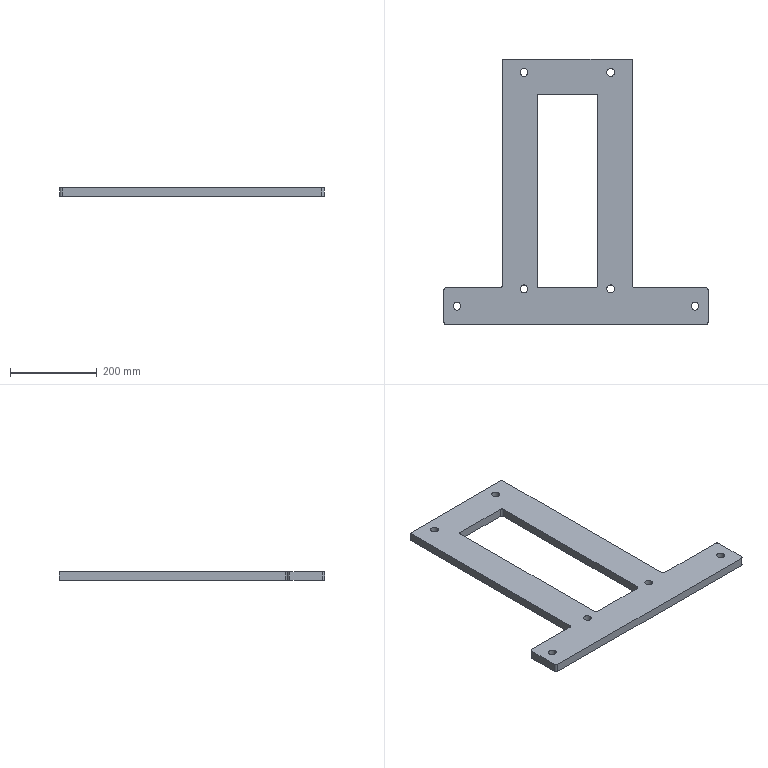Part | SolidWorks | features Extrusion 1 | 1 solid | 36 faces | box 610 x 612.5 x 20 mm | volume 2918678 mm3 | cylinder 22 | plane 14 | commonest cylinder face diameters 18 x12 10 x10
STEP:
#1=CARTESIAN_POINT('',(376.,82.5,20.));
#2=VERTEX_POINT('',#1);
#3=CARTESIAN_POINT('',(394.,82.5,20.));
#4=VERTEX_POINT('',#3);
#5=CARTESIAN_POINT('',(385.,82.5,20.));
#6=DIRECTION('',(0.,0.,1.));
#7=DIRECTION('',(1.,0.,0.));
#8=AXIS2_PLACEMENT_3D('',#5,#6,#7);
#9=CIRCLE('',#8,9.);
#10=EDGE_CURVE('',#2,#4,#9,.T.);
#11=ORIENTED_EDGE('',*,*,#10,.T.);
#12=CARTESIAN_POINT('',(394.,82.5,0.));
#13=VERTEX_POINT('',#12);
#14=CARTESIAN_POINT('',(394.,82.5,20.));
#15=DIRECTION('',(0.,0.,-1.));
#16=VECTOR('',#15,1000.);
#17=LINE('',#14,#16);
#18=EDGE_CURVE('',#4,#13,#17,.T.);
#19=ORIENTED_EDGE('',*,*,#18,.T.);
#20=CARTESIAN_POINT('',(376.,82.5,0.));
#21=VERTEX_POINT('',#20);
#22=CARTESIAN_POINT('',(385.,82.5,0.));
#23=DIRECTION('',(0.,0.,1.));
#24=DIRECTION('',(1.,0.,0.));
#25=AXIS2_PLACEMENT_3D('',#22,#23,#24);
#26=CIRCLE('',#25,9.);
#27=EDGE_CURVE('',#21,#13,#26,.T.);
#28=ORIENTED_EDGE('',*,*,#27,.F.);
#29=CARTESIAN_POINT('',(376.,82.5,20.));
#30=DIRECTION('',(0.,0.,-1.));
#31=VECTOR('',#30,1000.);
#32=LINE('',#29,#31);
#33=EDGE_CURVE('',#2,#21,#32,.T.);
#34=ORIENTED_EDGE('',*,*,#33,.F.);
#35=EDGE_LOOP('',(#11,#19,#28,#34));
#36=FACE_OUTER_BOUND('',#35,.T.);
#37=CARTESIAN_POINT('',(385.,82.5,20.));
#38=DIRECTION('',(0.,0.,-1.));
#39=DIRECTION('',(-1.,0.,0.));
#40=AXIS2_PLACEMENT_3D('',#37,#38,#39);
#41=CYLINDRICAL_SURFACE('',#40,9.);
#42=ADVANCED_FACE('',(#36),#41,.F.);
#43=CARTESIAN_POINT('',(176.,82.5,20.));
#44=VERTEX_POINT('',#43);
#45=CARTESIAN_POINT('',(194.,82.5,20.));
#46=VERTEX_POINT('',#45);
#47=CARTESIAN_POINT('',(185.,82.5,20.));
#48=DIRECTION('',(0.,0.,1.));
#49=DIRECTION('',(1.,0.,0.));
#50=AXIS2_PLACEMENT_3D('',#47,#48,#49);
#51=CIRCLE('',#50,9.);
#52=EDGE_CURVE('',#44,#46,#51,.T.);
#53=ORIENTED_EDGE('',*,*,#52,.T.);
#54=CARTESIAN_POINT('',(194.,82.5,0.));
#55=VERTEX_POINT('',#54);
#56=CARTESIAN_POINT('',(194.,82.5,20.));
#57=DIRECTION('',(0.,0.,-1.));
#58=VECTOR('',#57,1000.);
#59=LINE('',#56,#58);
#60=EDGE_CURVE('',#46,#55,#59,.T.);
#61=ORIENTED_EDGE('',*,*,#60,.T.);
#62=CARTESIAN_POINT('',(176.,82.5,0.));
#63=VERTEX_POINT('',#62);
#64=CARTESIAN_POINT('',(185.,82.5,0.));
#65=DIRECTION('',(0.,0.,1.));
#66=DIRECTION('',(1.,0.,0.));
#67=AXIS2_PLACEMENT_3D('',#64,#65,#66);
#68=CIRCLE('',#67,9.);
#69=EDGE_CURVE('',#63,#55,#68,.T.);
#70=ORIENTED_EDGE('',*,*,#69,.F.);
#71=CARTESIAN_POINT('',(176.,82.5,20.));
#72=DIRECTION('',(0.,0.,-1.));
#73=VECTOR('',#72,1000.);
#74=LINE('',#71,#73);
#75=EDGE_CURVE('',#44,#63,#74,.T.);
#76=ORIENTED_EDGE('',*,*,#75,.F.);
#77=EDGE_LOOP('',(#53,#61,#70,#76));
#78=FACE_OUTER_BOUND('',#77,.T.);
#79=CARTESIAN_POINT('',(185.,82.5,20.));
#80=DIRECTION('',(0.,0.,-1.));
#81=DIRECTION('',(-1.,0.,0.));
#82=AXIS2_PLACEMENT_3D('',#79,#80,#81);
#83=CYLINDRICAL_SURFACE('',#82,9.);
#84=ADVANCED_FACE('',(#78),#83,.F.);
#85=CARTESIAN_POINT('',(376.,582.5,20.));
#86=VERTEX_POINT('',#85);
#87=CARTESIAN_POINT('',(394.,582.5,20.));
#88=VERTEX_POINT('',#87);
#89=CARTESIAN_POINT('',(385.,582.5,20.));
#90=DIRECTION('',(0.,0.,1.));
#91=DIRECTION('',(1.,0.,0.));
#92=AXIS2_PLACEMENT_3D('',#89,#90,#91);
#93=CIRCLE('',#92,9.);
#94=EDGE_CURVE('',#86,#88,#93,.T.);
#95=ORIENTED_EDGE('',*,*,#94,.T.);
#96=CARTESIAN_POINT('',(394.,582.5,0.));
#97=VERTEX_POINT('',#96);
#98=CARTESIAN_POINT('',(394.,582.5,20.));
#99=DIRECTION('',(0.,0.,-1.));
#100=VECTOR('',#99,1000.);
#101=LINE('',#98,#100);
#102=EDGE_CURVE('',#88,#97,#101,.T.);
#103=ORIENTED_EDGE('',*,*,#102,.T.);
#104=CARTESIAN_POINT('',(376.,582.5,0.));
#105=VERTEX_POINT('',#104);
#106=CARTESIAN_POINT('',(385.,582.5,0.));
#107=DIRECTION('',(0.,0.,1.));
#108=DIRECTION('',(1.,0.,0.));
#109=AXIS2_PLACEMENT_3D('',#106,#107,#108);
#110=CIRCLE('',#109,9.);
#111=EDGE_CURVE('',#105,#97,#110,.T.);
#112=ORIENTED_EDGE('',*,*,#111,.F.);
#113=CARTESIAN_POINT('',(376.,582.5,20.));
#114=DIRECTION('',(0.,0.,-1.));
#115=VECTOR('',#114,1000.);
#116=LINE('',#113,#115);
#117=EDGE_CURVE('',#86,#105,#116,.T.);
#118=ORIENTED_EDGE('',*,*,#117,.F.);
#119=EDGE_LOOP('',(#95,#103,#112,#118));
#120=FACE_OUTER_BOUND('',#119,.T.);
#121=CARTESIAN_POINT('',(385.,582.5,20.));
#122=DIRECTION('',(0.,0.,-1.));
#123=DIRECTION('',(-1.,0.,0.));
#124=AXIS2_PLACEMENT_3D('',#121,#122,#123);
#125=CYLINDRICAL_SURFACE('',#124,9.);
#126=ADVANCED_FACE('',(#120),#125,.F.);
#127=CARTESIAN_POINT('',(176.,582.5,20.));
#128=VERTEX_POINT('',#127);
#129=CARTESIAN_POINT('',(194.,582.5,20.));
#130=VERTEX_POINT('',#129);
#131=CARTESIAN_POINT('',(185.,582.5,20.));
#132=DIRECTION('',(0.,0.,1.));
#133=DIRECTION('',(1.,0.,0.));
#134=AXIS2_PLACEMENT_3D('',#131,#132,#133);
#135=CIRCLE('',#134,9.);
#136=EDGE_CURVE('',#128,#130,#135,.T.);
#137=ORIENTED_EDGE('',*,*,#136,.T.);
#138=CARTESIAN_POINT('',(194.,582.5,0.));
#139=VERTEX_POINT('',#138);
#140=CARTESIAN_POINT('',(194.,582.5,20.));
#141=DIRECTION('',(0.,0.,-1.));
#142=VECTOR('',#141,1000.);
#143=LINE('',#140,#142);
#144=EDGE_CURVE('',#130,#139,#143,.T.);
#145=ORIENTED_EDGE('',*,*,#144,.T.);
#146=CARTESIAN_POINT('',(176.,582.5,0.));
#147=VERTEX_POINT('',#146);
#148=CARTESIAN_POINT('',(185.,582.5,0.));
#149=DIRECTION('',(0.,0.,1.));
#150=DIRECTION('',(1.,0.,0.));
#151=AXIS2_PLACEMENT_3D('',#148,#149,#150);
#152=CIRCLE('',#151,9.);
#153=EDGE_CURVE('',#147,#139,#152,.T.);
#154=ORIENTED_EDGE('',*,*,#153,.F.);
#155=CARTESIAN_POINT('',(176.,582.5,20.));
#156=DIRECTION('',(0.,0.,-1.));
#157=VECTOR('',#156,1000.);
#158=LINE('',#155,#157);
#159=EDGE_CURVE('',#128,#147,#158,.T.);
#160=ORIENTED_EDGE('',*,*,#159,.F.);
#161=EDGE_LOOP('',(#137,#145,#154,#160));
#162=FACE_OUTER_BOUND('',#161,.T.);
#163=CARTESIAN_POINT('',(185.,582.5,20.));
#164=DIRECTION('',(0.,0.,-1.));
#165=DIRECTION('',(-1.,0.,0.));
#166=AXIS2_PLACEMENT_3D('',#163,#164,#165);
#167=CYLINDRICAL_SURFACE('',#166,9.);
#168=ADVANCED_FACE('',(#162),#167,.F.);
#169=CARTESIAN_POINT('',(571.,42.5,20.));
#170=VERTEX_POINT('',#169);
#171=CARTESIAN_POINT('',(589.,42.5,20.));
#172=VERTEX_POINT('',#171);
#173=CARTESIAN_POINT('',(580.,42.5,20.));
#174=DIRECTION('',(0.,0.,1.));
#175=DIRECTION('',(1.,0.,0.));
#176=AXIS2_PLACEMENT_3D('',#173,#174,#175);
#177=CIRCLE('',#176,9.);
#178=EDGE_CURVE('',#170,#172,#177,.T.);
#179=ORIENTED_EDGE('',*,*,#178,.T.);
#180=CARTESIAN_POINT('',(589.,42.5,0.));
#181=VERTEX_POINT('',#180);
#182=CARTESIAN_POINT('',(589.,42.5,20.));
#183=DIRECTION('',(0.,0.,-1.));
#184=VECTOR('',#183,1000.);
#185=LINE('',#182,#184);
#186=EDGE_CURVE('',#172,#181,#185,.T.);
#187=ORIENTED_EDGE('',*,*,#186,.T.);
#188=CARTESIAN_POINT('',(571.,42.5,0.));
#189=VERTEX_POINT('',#188);
#190=CARTESIAN_POINT('',(580.,42.5,0.));
#191=DIRECTION('',(0.,0.,1.));
#192=DIRECTION('',(1.,0.,0.));
#193=AXIS2_PLACEMENT_3D('',#190,#191,#192);
#194=CIRCLE('',#193,9.);
#195=EDGE_CURVE('',#189,#181,#194,.T.);
#196=ORIENTED_EDGE('',*,*,#195,.F.);
#197=CARTESIAN_POINT('',(571.,42.5,20.));
#198=DIRECTION('',(0.,0.,-1.));
#199=VECTOR('',#198,1000.);
#200=LINE('',#197,#199);
#201=EDGE_CURVE('',#170,#189,#200,.T.);
#202=ORIENTED_EDGE('',*,*,#201,.F.);
#203=EDGE_LOOP('',(#179,#187,#196,#202));
#204=FACE_OUTER_BOUND('',#203,.T.);
#205=CARTESIAN_POINT('',(580.,42.5,20.));
#206=DIRECTION('',(0.,0.,-1.));
#207=DIRECTION('',(-1.,0.,0.));
#208=AXIS2_PLACEMENT_3D('',#205,#206,#207);
#209=CYLINDRICAL_SURFACE('',#208,9.);
#210=ADVANCED_FACE('',(#204),#209,.F.);
#211=CARTESIAN_POINT('',(21.,42.5,20.));
#212=VERTEX_POINT('',#211);
#213=CARTESIAN_POINT('',(39.,42.5,20.));
#214=VERTEX_POINT('',#213);
#215=CARTESIAN_POINT('',(30.,42.5,20.));
#216=DIRECTION('',(0.,0.,1.));
#217=DIRECTION('',(1.,0.,0.));
#218=AXIS2_PLACEMENT_3D('',#215,#216,#217);
#219=CIRCLE('',#218,9.);
#220=EDGE_CURVE('',#212,#214,#219,.T.);
#221=ORIENTED_EDGE('',*,*,#220,.T.);
#222=CARTESIAN_POINT('',(39.,42.5,0.));
#223=VERTEX_POINT('',#222);
#224=CARTESIAN_POINT('',(39.,42.5,20.));
#225=DIRECTION('',(0.,0.,-1.));
#226=VECTOR('',#225,1000.);
#227=LINE('',#224,#226);
#228=EDGE_CURVE('',#214,#223,#227,.T.);
#229=ORIENTED_EDGE('',*,*,#228,.T.);
#230=CARTESIAN_POINT('',(21.,42.5,0.));
#231=VERTEX_POINT('',#230);
#232=CARTESIAN_POINT('',(30.,42.5,0.));
#233=DIRECTION('',(0.,0.,1.));
#234=DIRECTION('',(1.,0.,0.));
#235=AXIS2_PLACEMENT_3D('',#232,#233,#234);
#236=CIRCLE('',#235,9.);
#237=EDGE_CURVE('',#231,#223,#236,.T.);
#238=ORIENTED_EDGE('',*,*,#237,.F.);
#239=CARTESIAN_POINT('',(21.,42.5,20.));
#240=DIRECTION('',(0.,0.,-1.));
#241=VECTOR('',#240,1000.);
#242=LINE('',#239,#241);
#243=EDGE_CURVE('',#212,#231,#242,.T.);
#244=ORIENTED_EDGE('',*,*,#243,.F.);
#245=EDGE_LOOP('',(#221,#229,#238,#244));
#246=FACE_OUTER_BOUND('',#245,.T.);
#247=CARTESIAN_POINT('',(30.,42.5,20.));
#248=DIRECTION('',(0.,0.,-1.));
#249=DIRECTION('',(-1.,0.,0.));
#250=AXIS2_PLACEMENT_3D('',#247,#248,#249);
#251=CYLINDRICAL_SURFACE('',#250,9.);
#252=ADVANCED_FACE('',(#246),#251,.F.);
#253=CARTESIAN_POINT('',(435.,612.5,20.));
#254=VERTEX_POINT('',#253);
#255=CARTESIAN_POINT('',(135.,612.5,20.));
#256=VERTEX_POINT('',#255);
#257=CARTESIAN_POINT('',(435.,612.5,20.));
#258=DIRECTION('',(-1.,0.,0.));
#259=VECTOR('',#258,1000.);
#260=LINE('',#257,#259);
#261=EDGE_CURVE('',#254,#256,#260,.T.);
#262=ORIENTED_EDGE('',*,*,#261,.T.);
#263=CARTESIAN_POINT('',(135.,90.,20.));
#264=VERTEX_POINT('',#263);
#265=CARTESIAN_POINT('',(135.,612.5,20.));
#266=DIRECTION('',(0.,-1.,0.));
#267=VECTOR('',#266,1000.);
#268=LINE('',#265,#267);
#269=EDGE_CURVE('',#256,#264,#268,.T.);
#270=ORIENTED_EDGE('',*,*,#269,.T.);
#271=CARTESIAN_POINT('',(130.,85.,20.));
#272=VERTEX_POINT('',#271);
#273=CARTESIAN_POINT('',(130.,90.,20.));
#274=DIRECTION('',(0.,0.,-1.));
#275=DIRECTION('',(-1.,0.,0.));
#276=AXIS2_PLACEMENT_3D('',#273,#274,#275);
#277=CIRCLE('',#276,5.);
#278=EDGE_CURVE('',#264,#272,#277,.T.);
#279=ORIENTED_EDGE('',*,*,#278,.T.);
#280=CARTESIAN_POINT('',(5.,85.,20.));
#281=VERTEX_POINT('',#280);
#282=CARTESIAN_POINT('',(130.,85.,20.));
#283=DIRECTION('',(-1.,0.,0.));
#284=VECTOR('',#283,1000.);
#285=LINE('',#282,#284);
#286=EDGE_CURVE('',#272,#281,#285,.T.);
#287=ORIENTED_EDGE('',*,*,#286,.T.);
#288=CARTESIAN_POINT('',(0.,80.,20.));
#289=VERTEX_POINT('',#288);
#290=CARTESIAN_POINT('',(5.,80.,20.));
#291=DIRECTION('',(0.,0.,1.));
#292=DIRECTION('',(1.,0.,0.));
#293=AXIS2_PLACEMENT_3D('',#290,#291,#292);
#294=CIRCLE('',#293,5.);
#295=EDGE_CURVE('',#281,#289,#294,.T.);
#296=ORIENTED_EDGE('',*,*,#295,.T.);
#297=CARTESIAN_POINT('',(0.,5.,20.));
#298=VERTEX_POINT('',#297);
#299=CARTESIAN_POINT('',(0.,80.,20.));
#300=DIRECTION('',(0.,-1.,0.));
#301=VECTOR('',#300,1000.);
#302=LINE('',#299,#301);
#303=EDGE_CURVE('',#289,#298,#302,.T.);
#304=ORIENTED_EDGE('',*,*,#303,.T.);
#305=CARTESIAN_POINT('',(5.,0.,20.));
#306=VERTEX_POINT('',#305);
#307=CARTESIAN_POINT('',(5.,5.,20.));
#308=DIRECTION('',(0.,0.,1.));
#309=DIRECTION('',(-1.,0.,0.));
#310=AXIS2_PLACEMENT_3D('',#307,#308,#309);
#311=CIRCLE('',#310,5.);
#312=EDGE_CURVE('',#298,#306,#311,.T.);
#313=ORIENTED_EDGE('',*,*,#312,.T.);
#314=CARTESIAN_POINT('',(605.,0.,20.));
#315=VERTEX_POINT('',#314);
#316=CARTESIAN_POINT('',(5.,0.,20.));
#317=DIRECTION('',(1.,0.,0.));
#318=VECTOR('',#317,1000.);
#319=LINE('',#316,#318);
#320=EDGE_CURVE('',#306,#315,#319,.T.);
#321=ORIENTED_EDGE('',*,*,#320,.T.);
#322=CARTESIAN_POINT('',(610.,5.,20.));
#323=VERTEX_POINT('',#322);
#324=CARTESIAN_POINT('',(605.,5.,20.));
#325=DIRECTION('',(0.,0.,1.));
#326=DIRECTION('',(1.,0.,0.));
#327=AXIS2_PLACEMENT_3D('',#324,#325,#326);
#328=CIRCLE('',#327,5.);
#329=EDGE_CURVE('',#315,#323,#328,.T.);
#330=ORIENTED_EDGE('',*,*,#329,.T.);
#331=CARTESIAN_POINT('',(610.,80.,20.));
#332=VERTEX_POINT('',#331);
#333=CARTESIAN_POINT('',(610.,5.,20.));
#334=DIRECTION('',(0.,1.,0.));
#335=VECTOR('',#334,1000.);
#336=LINE('',#333,#335);
#337=EDGE_CURVE('',#323,#332,#336,.T.);
#338=ORIENTED_EDGE('',*,*,#337,.T.);
#339=CARTESIAN_POINT('',(605.,85.,20.));
#340=VERTEX_POINT('',#339);
#341=CARTESIAN_POINT('',(605.,80.,20.));
#342=DIRECTION('',(0.,0.,1.));
#343=DIRECTION('',(1.,0.,0.));
#344=AXIS2_PLACEMENT_3D('',#341,#342,#343);
#345=CIRCLE('',#344,5.);
#346=EDGE_CURVE('',#332,#340,#345,.T.);
#347=ORIENTED_EDGE('',*,*,#346,.T.);
#348=CARTESIAN_POINT('',(440.,85.,20.));
#349=VERTEX_POINT('',#348);
#350=CARTESIAN_POINT('',(605.,85.,20.));
#351=DIRECTION('',(-1.,0.,0.));
#352=VECTOR('',#351,1000.);
#353=LINE('',#350,#352);
#354=EDGE_CURVE('',#340,#349,#353,.T.);
#355=ORIENTED_EDGE('',*,*,#354,.T.);
#356=CARTESIAN_POINT('',(435.,90.,20.));
#357=VERTEX_POINT('',#356);
#358=CARTESIAN_POINT('',(440.,90.,20.));
#359=DIRECTION('',(0.,0.,-1.));
#360=DIRECTION('',(-1.,0.,0.));
#361=AXIS2_PLACEMENT_3D('',#358,#359,#360);
#362=CIRCLE('',#361,5.);
#363=EDGE_CURVE('',#349,#357,#362,.T.);
#364=ORIENTED_EDGE('',*,*,#363,.T.);
#365=CARTESIAN_POINT('',(435.,90.,20.));
#366=DIRECTION('',(0.,1.,0.));
#367=VECTOR('',#366,1000.);
#368=LINE('',#365,#367);
#369=EDGE_CURVE('',#357,#254,#368,.T.);
#370=ORIENTED_EDGE('',*,*,#369,.T.);
#371=EDGE_LOOP('',(#262,#270,#279,#287,#296,#304,#313,#321,#330,#338,#347,#355,#364,#370));
#372=FACE_OUTER_BOUND('',#371,.T.);
#373=CARTESIAN_POINT('',(220.,532.5,20.));
#374=VERTEX_POINT('',#373);
#375=CARTESIAN_POINT('',(215.,527.5,20.));
#376=VERTEX_POINT('',#375);
#377=CARTESIAN_POINT('',(220.,527.5,20.));
#378=DIRECTION('',(0.,0.,1.));
#379=DIRECTION('',(-1.,0.,0.));
#380=AXIS2_PLACEMENT_3D('',#377,#378,#379);
#381=CIRCLE('',#380,5.);
#382=EDGE_CURVE('',#374,#376,#381,.T.);
#383=ORIENTED_EDGE('',*,*,#382,.F.);
#384=CARTESIAN_POINT('',(350.,532.5,20.));
#385=VERTEX_POINT('',#384);
#386=CARTESIAN_POINT('',(220.,532.5,20.));
#387=DIRECTION('',(-1.,0.,0.));
#388=VECTOR('',#387,1000.);
#389=LINE('',#386,#388);
#390=EDGE_CURVE('',#385,#374,#389,.T.);
#391=ORIENTED_EDGE('',*,*,#390,.F.);
#392=CARTESIAN_POINT('',(355.,527.5,20.));
#393=VERTEX_POINT('',#392);
#394=CARTESIAN_POINT('',(350.,527.5,20.));
#395=DIRECTION('',(0.,0.,1.));
#396=DIRECTION('',(-1.,0.,0.));
#397=AXIS2_PLACEMENT_3D('',#394,#395,#396);
#398=CIRCLE('',#397,5.);
#399=EDGE_CURVE('',#393,#385,#398,.T.);
#400=ORIENTED_EDGE('',*,*,#399,.F.);
#401=CARTESIAN_POINT('',(355.,90.,20.));
#402=VERTEX_POINT('',#401);
#403=CARTESIAN_POINT('',(355.,90.,20.));
#404=DIRECTION('',(0.,1.,0.));
#405=VECTOR('',#404,1000.);
#406=LINE('',#403,#405);
#407=EDGE_CURVE('',#402,#393,#406,.T.);
#408=ORIENTED_EDGE('',*,*,#407,.F.);
#409=CARTESIAN_POINT('',(350.,85.,20.));
#410=VERTEX_POINT('',#409);
#411=CARTESIAN_POINT('',(350.,90.,20.));
#412=DIRECTION('',(0.,0.,1.));
#413=DIRECTION('',(1.,0.,0.));
#414=AXIS2_PLACEMENT_3D('',#411,#412,#413);
#415=CIRCLE('',#414,5.);
#416=EDGE_CURVE('',#410,#402,#415,.T.);
#417=ORIENTED_EDGE('',*,*,#416,.F.);
#418=CARTESIAN_POINT('',(220.,85.,20.));
#419=VERTEX_POINT('',#418);
#420=CARTESIAN_POINT('',(220.,85.,20.));
#421=DIRECTION('',(1.,0.,0.));
#422=VECTOR('',#421,1000.);
#423=LINE('',#420,#422);
#424=EDGE_CURVE('',#419,#410,#423,.T.);
#425=ORIENTED_EDGE('',*,*,#424,.F.);
#426=CARTESIAN_POINT('',(215.,90.,20.));
#427=VERTEX_POINT('',#426);
#428=CARTESIAN_POINT('',(220.,90.,20.));
#429=DIRECTION('',(0.,0.,1.));
#430=DIRECTION('',(-1.,0.,0.));
#431=AXIS2_PLACEMENT_3D('',#428,#429,#430);
#432=CIRCLE('',#431,5.);
#433=EDGE_CURVE('',#427,#419,#432,.T.);
#434=ORIENTED_EDGE('',*,*,#433,.F.);
#435=CARTESIAN_POINT('',(215.,90.,20.));
#436=DIRECTION('',(0.,-1.,0.));
#437=VECTOR('',#436,1000.);
#438=LINE('',#435,#437);
#439=EDGE_CURVE('',#376,#427,#438,.T.);
#440=ORIENTED_EDGE('',*,*,#439,.F.);
#441=EDGE_LOOP('',(#383,#391,#400,#408,#417,#425,#434,#440));
#442=FACE_BOUND('',#441,.T.);
#443=ORIENTED_EDGE('',*,*,#220,.F.);
#444=CARTESIAN_POINT('',(30.,42.5,20.));
#445=DIRECTION('',(0.,0.,1.));
#446=DIRECTION('',(1.,0.,0.));
#447=AXIS2_PLACEMENT_3D('',#444,#445,#446);
#448=CIRCLE('',#447,9.);
#449=EDGE_CURVE('',#214,#212,#448,.T.);
#450=ORIENTED_EDGE('',*,*,#449,.F.);
#451=EDGE_LOOP('',(#443,#450));
#452=FACE_BOUND('',#451,.T.);
#453=ORIENTED_EDGE('',*,*,#178,.F.);
#454=CARTESIAN_POINT('',(580.,42.5,20.));
#455=DIRECTION('',(0.,0.,1.));
#456=DIRECTION('',(1.,0.,0.));
#457=AXIS2_PLACEMENT_3D('',#454,#455,#456);
#458=CIRCLE('',#457,9.);
#459=EDGE_CURVE('',#172,#170,#458,.T.);
#460=ORIENTED_EDGE('',*,*,#459,.F.);
#461=EDGE_LOOP('',(#453,#460));
#462=FACE_BOUND('',#461,.T.);
#463=ORIENTED_EDGE('',*,*,#136,.F.);
#464=CARTESIAN_POINT('',(185.,582.5,20.));
#465=DIRECTION('',(0.,0.,1.));
#466=DIRECTION('',(1.,0.,0.));
#467=AXIS2_PLACEMENT_3D('',#464,#465,#466);
#468=CIRCLE('',#467,9.);
#469=EDGE_CURVE('',#130,#128,#468,.T.);
#470=ORIENTED_EDGE('',*,*,#469,.F.);
#471=EDGE_LOOP('',(#463,#470));
#472=FACE_BOUND('',#471,.T.);
#473=ORIENTED_EDGE('',*,*,#94,.F.);
#474=CARTESIAN_POINT('',(385.,582.5,20.));
#475=DIRECTION('',(0.,0.,1.));
#476=DIRECTION('',(1.,0.,0.));
#477=AXIS2_PLACEMENT_3D('',#474,#475,#476);
#478=CIRCLE('',#477,9.);
#479=EDGE_CURVE('',#88,#86,#478,.T.);
#480=ORIENTED_EDGE('',*,*,#479,.F.);
#481=EDGE_LOOP('',(#473,#480));
#482=FACE_BOUND('',#481,.T.);
#483=ORIENTED_EDGE('',*,*,#52,.F.);
#484=CARTESIAN_POINT('',(185.,82.5,20.));
#485=DIRECTION('',(0.,0.,1.));
#486=DIRECTION('',(1.,0.,0.));
#487=AXIS2_PLACEMENT_3D('',#484,#485,#486);
#488=CIRCLE('',#487,9.);
#489=EDGE_CURVE('',#46,#44,#488,.T.);
#490=ORIENTED_EDGE('',*,*,#489,.F.);
#491=EDGE_LOOP('',(#483,#490));
#492=FACE_BOUND('',#491,.T.);
#493=ORIENTED_EDGE('',*,*,#10,.F.);
#494=CARTESIAN_POINT('',(385.,82.5,20.));
#495=DIRECTION('',(0.,0.,1.));
#496=DIRECTION('',(1.,0.,0.));
#497=AXIS2_PLACEMENT_3D('',#494,#495,#496);
#498=CIRCLE('',#497,9.);
#499=EDGE_CURVE('',#4,#2,#498,.T.);
#500=ORIENTED_EDGE('',*,*,#499,.F.);
#501=EDGE_LOOP('',(#493,#500));
#502=FACE_BOUND('',#501,.T.);
#503=CARTESIAN_POINT('',(130.,90.,20.));
#504=DIRECTION('',(0.,0.,-1.));
#505=DIRECTION('',(-1.,0.,0.));
#506=AXIS2_PLACEMENT_3D('',#503,#504,#505);
#507=PLANE('',#506);
#508=ADVANCED_FACE('',(#372,#442,#452,#462,#472,#482,#492,#502),#507,.F.);
#509=ORIENTED_EDGE('',*,*,#69,.T.);
#510=CARTESIAN_POINT('',(185.,82.5,0.));
#511=DIRECTION('',(0.,0.,1.));
#512=DIRECTION('',(1.,0.,0.));
#513=AXIS2_PLACEMENT_3D('',#510,#511,#512);
#514=CIRCLE('',#513,9.);
#515=EDGE_CURVE('',#55,#63,#514,.T.);
#516=ORIENTED_EDGE('',*,*,#515,.T.);
#517=EDGE_LOOP('',(#509,#516));
#518=FACE_BOUND('',#517,.T.);
#519=ORIENTED_EDGE('',*,*,#153,.T.);
#520=CARTESIAN_POINT('',(185.,582.5,0.));
#521=DIRECTION('',(0.,0.,1.));
#522=DIRECTION('',(1.,0.,0.));
#523=AXIS2_PLACEMENT_3D('',#520,#521,#522);
#524=CIRCLE('',#523,9.);
#525=EDGE_CURVE('',#139,#147,#524,.T.);
#526=ORIENTED_EDGE('',*,*,#525,.T.);
#527=EDGE_LOOP('',(#519,#526));
#528=FACE_BOUND('',#527,.T.);
#529=ORIENTED_EDGE('',*,*,#237,.T.);
#530=CARTESIAN_POINT('',(30.,42.5,0.));
#531=DIRECTION('',(0.,0.,1.));
#532=DIRECTION('',(1.,0.,0.));
#533=AXIS2_PLACEMENT_3D('',#530,#531,#532);
#534=CIRCLE('',#533,9.);
#535=EDGE_CURVE('',#223,#231,#534,.T.);
#536=ORIENTED_EDGE('',*,*,#535,.T.);
#537=EDGE_LOOP('',(#529,#536));
#538=FACE_BOUND('',#537,.T.);
#539=CARTESIAN_POINT('',(435.,612.5,0.));
#540=VERTEX_POINT('',#539);
#541=CARTESIAN_POINT('',(135.,612.5,0.));
#542=VERTEX_POINT('',#541);
#543=CARTESIAN_POINT('',(435.,612.5,0.));
#544=DIRECTION('',(-1.,0.,0.));
#545=VECTOR('',#544,1000.);
#546=LINE('',#543,#545);
#547=EDGE_CURVE('',#540,#542,#546,.T.);
#548=ORIENTED_EDGE('',*,*,#547,.F.);
#549=CARTESIAN_POINT('',(435.,90.,0.));
#550=VERTEX_POINT('',#549);
#551=CARTESIAN_POINT('',(435.,90.,0.));
#552=DIRECTION('',(0.,1.,0.));
#553=VECTOR('',#552,1000.);
#554=LINE('',#551,#553);
#555=EDGE_CURVE('',#550,#540,#554,.T.);
#556=ORIENTED_EDGE('',*,*,#555,.F.);
#557=CARTESIAN_POINT('',(440.,85.,0.));
#558=VERTEX_POINT('',#557);
#559=CARTESIAN_POINT('',(440.,90.,0.));
#560=DIRECTION('',(0.,0.,-1.));
#561=DIRECTION('',(-1.,0.,0.));
#562=AXIS2_PLACEMENT_3D('',#559,#560,#561);
#563=CIRCLE('',#562,5.);
#564=EDGE_CURVE('',#558,#550,#563,.T.);
#565=ORIENTED_EDGE('',*,*,#564,.F.);
#566=CARTESIAN_POINT('',(605.,85.,0.));
#567=VERTEX_POINT('',#566);
#568=CARTESIAN_POINT('',(605.,85.,0.));
#569=DIRECTION('',(-1.,0.,0.));
#570=VECTOR('',#569,1000.);
#571=LINE('',#568,#570);
#572=EDGE_CURVE('',#567,#558,#571,.T.);
#573=ORIENTED_EDGE('',*,*,#572,.F.);
#574=CARTESIAN_POINT('',(610.,80.,0.));
#575=VERTEX_POINT('',#574);
#576=CARTESIAN_POINT('',(605.,80.,0.));
#577=DIRECTION('',(0.,0.,1.));
#578=DIRECTION('',(1.,0.,0.));
#579=AXIS2_PLACEMENT_3D('',#576,#577,#578);
#580=CIRCLE('',#579,5.);
#581=EDGE_CURVE('',#575,#567,#580,.T.);
#582=ORIENTED_EDGE('',*,*,#581,.F.);
#583=CARTESIAN_POINT('',(610.,5.,0.));
#584=VERTEX_POINT('',#583);
#585=CARTESIAN_POINT('',(610.,5.,0.));
#586=DIRECTION('',(0.,1.,0.));
#587=VECTOR('',#586,1000.);
#588=LINE('',#585,#587);
#589=EDGE_CURVE('',#584,#575,#588,.T.);
#590=ORIENTED_EDGE('',*,*,#589,.F.);
#591=CARTESIAN_POINT('',(605.,0.,0.));
#592=VERTEX_POINT('',#591);
#593=CARTESIAN_POINT('',(605.,5.,0.));
#594=DIRECTION('',(0.,0.,1.));
#595=DIRECTION('',(1.,0.,0.));
#596=AXIS2_PLACEMENT_3D('',#593,#594,#595);
#597=CIRCLE('',#596,5.);
#598=EDGE_CURVE('',#592,#584,#597,.T.);
#599=ORIENTED_EDGE('',*,*,#598,.F.);
#600=CARTESIAN_POINT('',(5.,0.,0.));
#601=VERTEX_POINT('',#600);
#602=CARTESIAN_POINT('',(5.,0.,0.));
#603=DIRECTION('',(1.,0.,0.));
#604=VECTOR('',#603,1000.);
#605=LINE('',#602,#604);
#606=EDGE_CURVE('',#601,#592,#605,.T.);
#607=ORIENTED_EDGE('',*,*,#606,.F.);
#608=CARTESIAN_POINT('',(0.,5.,0.));
#609=VERTEX_POINT('',#608);
#610=CARTESIAN_POINT('',(5.,5.,0.));
#611=DIRECTION('',(0.,0.,1.));
#612=DIRECTION('',(-1.,0.,0.));
#613=AXIS2_PLACEMENT_3D('',#610,#611,#612);
#614=CIRCLE('',#613,5.);
#615=EDGE_CURVE('',#609,#601,#614,.T.);
#616=ORIENTED_EDGE('',*,*,#615,.F.);
#617=CARTESIAN_POINT('',(0.,80.,0.));
#618=VERTEX_POINT('',#617);
#619=CARTESIAN_POINT('',(0.,80.,0.));
#620=DIRECTION('',(0.,-1.,0.));
#621=VECTOR('',#620,1000.);
#622=LINE('',#619,#621);
#623=EDGE_CURVE('',#618,#609,#622,.T.);
#624=ORIENTED_EDGE('',*,*,#623,.F.);
#625=CARTESIAN_POINT('',(5.,85.,0.));
#626=VERTEX_POINT('',#625);
#627=CARTESIAN_POINT('',(5.,80.,0.));
#628=DIRECTION('',(0.,0.,1.));
#629=DIRECTION('',(1.,0.,0.));
#630=AXIS2_PLACEMENT_3D('',#627,#628,#629);
#631=CIRCLE('',#630,5.);
#632=EDGE_CURVE('',#626,#618,#631,.T.);
#633=ORIENTED_EDGE('',*,*,#632,.F.);
#634=CARTESIAN_POINT('',(130.,85.,0.));
#635=VERTEX_POINT('',#634);
#636=CARTESIAN_POINT('',(130.,85.,0.));
#637=DIRECTION('',(-1.,0.,0.));
#638=VECTOR('',#637,1000.);
#639=LINE('',#636,#638);
#640=EDGE_CURVE('',#635,#626,#639,.T.);
#641=ORIENTED_EDGE('',*,*,#640,.F.);
#642=CARTESIAN_POINT('',(135.,90.,0.));
#643=VERTEX_POINT('',#642);
#644=CARTESIAN_POINT('',(130.,90.,0.));
#645=DIRECTION('',(0.,0.,-1.));
#646=DIRECTION('',(-1.,0.,0.));
#647=AXIS2_PLACEMENT_3D('',#644,#645,#646);
#648=CIRCLE('',#647,5.);
#649=EDGE_CURVE('',#643,#635,#648,.T.);
#650=ORIENTED_EDGE('',*,*,#649,.F.);
#651=CARTESIAN_POINT('',(135.,612.5,0.));
#652=DIRECTION('',(0.,-1.,0.));
#653=VECTOR('',#652,1000.);
#654=LINE('',#651,#653);
#655=EDGE_CURVE('',#542,#643,#654,.T.);
#656=ORIENTED_EDGE('',*,*,#655,.F.);
#657=EDGE_LOOP('',(#548,#556,#565,#573,#582,#590,#599,#607,#616,#624,#633,#641,#650,#656));
#658=FACE_OUTER_BOUND('',#657,.T.);
#659=CARTESIAN_POINT('',(350.,532.5,0.));
#660=VERTEX_POINT('',#659);
#661=CARTESIAN_POINT('',(220.,532.5,0.));
#662=VERTEX_POINT('',#661);
#663=CARTESIAN_POINT('',(220.,532.5,0.));
#664=DIRECTION('',(-1.,0.,0.));
#665=VECTOR('',#664,1000.);
#666=LINE('',#663,#665);
#667=EDGE_CURVE('',#660,#662,#666,.T.);
#668=ORIENTED_EDGE('',*,*,#667,.T.);
#669=CARTESIAN_POINT('',(215.,527.5,0.));
#670=VERTEX_POINT('',#669);
#671=CARTESIAN_POINT('',(220.,527.5,0.));
#672=DIRECTION('',(0.,0.,1.));
#673=DIRECTION('',(-1.,0.,0.));
#674=AXIS2_PLACEMENT_3D('',#671,#672,#673);
#675=CIRCLE('',#674,5.);
#676=EDGE_CURVE('',#662,#670,#675,.T.);
#677=ORIENTED_EDGE('',*,*,#676,.T.);
#678=CARTESIAN_POINT('',(215.,90.,0.));
#679=VERTEX_POINT('',#678);
#680=CARTESIAN_POINT('',(215.,90.,0.));
#681=DIRECTION('',(0.,-1.,0.));
#682=VECTOR('',#681,1000.);
#683=LINE('',#680,#682);
#684=EDGE_CURVE('',#670,#679,#683,.T.);
#685=ORIENTED_EDGE('',*,*,#684,.T.);
#686=CARTESIAN_POINT('',(220.,85.,0.));
#687=VERTEX_POINT('',#686);
#688=CARTESIAN_POINT('',(220.,90.,0.));
#689=DIRECTION('',(0.,0.,1.));
#690=DIRECTION('',(-1.,0.,0.));
#691=AXIS2_PLACEMENT_3D('',#688,#689,#690);
#692=CIRCLE('',#691,5.);
#693=EDGE_CURVE('',#679,#687,#692,.T.);
#694=ORIENTED_EDGE('',*,*,#693,.T.);
#695=CARTESIAN_POINT('',(350.,85.,0.));
#696=VERTEX_POINT('',#695);
#697=CARTESIAN_POINT('',(220.,85.,0.));
#698=DIRECTION('',(1.,0.,0.));
#699=VECTOR('',#698,1000.);
#700=LINE('',#697,#699);
#701=EDGE_CURVE('',#687,#696,#700,.T.);
#702=ORIENTED_EDGE('',*,*,#701,.T.);
#703=CARTESIAN_POINT('',(355.,90.,0.));
#704=VERTEX_POINT('',#703);
#705=CARTESIAN_POINT('',(350.,90.,0.));
#706=DIRECTION('',(0.,0.,1.));
#707=DIRECTION('',(1.,0.,0.));
#708=AXIS2_PLACEMENT_3D('',#705,#706,#707);
#709=CIRCLE('',#708,5.);
#710=EDGE_CURVE('',#696,#704,#709,.T.);
#711=ORIENTED_EDGE('',*,*,#710,.T.);
#712=CARTESIAN_POINT('',(355.,527.5,0.));
#713=VERTEX_POINT('',#712);
#714=CARTESIAN_POINT('',(355.,90.,0.));
#715=DIRECTION('',(0.,1.,0.));
#716=VECTOR('',#715,1000.);
#717=LINE('',#714,#716);
#718=EDGE_CURVE('',#704,#713,#717,.T.);
#719=ORIENTED_EDGE('',*,*,#718,.T.);
#720=CARTESIAN_POINT('',(350.,527.5,0.));
#721=DIRECTION('',(0.,0.,1.));
#722=DIRECTION('',(-1.,0.,0.));
#723=AXIS2_PLACEMENT_3D('',#720,#721,#722);
#724=CIRCLE('',#723,5.);
#725=EDGE_CURVE('',#713,#660,#724,.T.);
#726=ORIENTED_EDGE('',*,*,#725,.T.);
#727=EDGE_LOOP('',(#668,#677,#685,#694,#702,#711,#719,#726));
#728=FACE_BOUND('',#727,.T.);
#729=ORIENTED_EDGE('',*,*,#195,.T.);
#730=CARTESIAN_POINT('',(580.,42.5,0.));
#731=DIRECTION('',(0.,0.,1.));
#732=DIRECTION('',(1.,0.,0.));
#733=AXIS2_PLACEMENT_3D('',#730,#731,#732);
#734=CIRCLE('',#733,9.);
#735=EDGE_CURVE('',#181,#189,#734,.T.);
#736=ORIENTED_EDGE('',*,*,#735,.T.);
#737=EDGE_LOOP('',(#729,#736));
#738=FACE_BOUND('',#737,.T.);
#739=ORIENTED_EDGE('',*,*,#111,.T.);
#740=CARTESIAN_POINT('',(385.,582.5,0.));
#741=DIRECTION('',(0.,0.,1.));
#742=DIRECTION('',(1.,0.,0.));
#743=AXIS2_PLACEMENT_3D('',#740,#741,#742);
#744=CIRCLE('',#743,9.);
#745=EDGE_CURVE('',#97,#105,#744,.T.);
#746=ORIENTED_EDGE('',*,*,#745,.T.);
#747=EDGE_LOOP('',(#739,#746));
#748=FACE_BOUND('',#747,.T.);
#749=ORIENTED_EDGE('',*,*,#27,.T.);
#750=CARTESIAN_POINT('',(385.,82.5,0.));
#751=DIRECTION('',(0.,0.,1.));
#752=DIRECTION('',(1.,0.,0.));
#753=AXIS2_PLACEMENT_3D('',#750,#751,#752);
#754=CIRCLE('',#753,9.);
#755=EDGE_CURVE('',#13,#21,#754,.T.);
#756=ORIENTED_EDGE('',*,*,#755,.T.);
#757=EDGE_LOOP('',(#749,#756));
#758=FACE_BOUND('',#757,.T.);
#759=CARTESIAN_POINT('',(130.,90.,0.));
#760=DIRECTION('',(0.,0.,-1.));
#761=DIRECTION('',(-1.,0.,0.));
#762=AXIS2_PLACEMENT_3D('',#759,#760,#761);
#763=PLANE('',#762);
#764=ADVANCED_FACE('',(#518,#528,#538,#658,#728,#738,#748,#758),#763,.T.);
#765=ORIENTED_EDGE('',*,*,#547,.T.);
#766=CARTESIAN_POINT('',(135.,612.5,20.));
#767=DIRECTION('',(0.,0.,-1.));
#768=VECTOR('',#767,1000.);
#769=LINE('',#766,#768);
#770=EDGE_CURVE('',#256,#542,#769,.T.);
#771=ORIENTED_EDGE('',*,*,#770,.F.);
#772=ORIENTED_EDGE('',*,*,#261,.F.);
#773=CARTESIAN_POINT('',(435.,612.5,20.));
#774=DIRECTION('',(0.,0.,-1.));
#775=VECTOR('',#774,1000.);
#776=LINE('',#773,#775);
#777=EDGE_CURVE('',#254,#540,#776,.T.);
#778=ORIENTED_EDGE('',*,*,#777,.T.);
#779=EDGE_LOOP('',(#765,#771,#772,#778));
#780=FACE_OUTER_BOUND('',#779,.T.);
#781=CARTESIAN_POINT('',(435.,612.5,20.));
#782=DIRECTION('',(0.,-1.,0.));
#783=DIRECTION('',(0.,0.,-1.));
#784=AXIS2_PLACEMENT_3D('',#781,#782,#783);
#785=PLANE('',#784);
#786=ADVANCED_FACE('',(#780),#785,.F.);
#787=ORIENTED_EDGE('',*,*,#655,.T.);
#788=CARTESIAN_POINT('',(135.,90.,20.));
#789=DIRECTION('',(0.,0.,-1.));
#790=VECTOR('',#789,1000.);
#791=LINE('',#788,#790);
#792=EDGE_CURVE('',#264,#643,#791,.T.);
#793=ORIENTED_EDGE('',*,*,#792,.F.);
#794=ORIENTED_EDGE('',*,*,#269,.F.);
#795=ORIENTED_EDGE('',*,*,#770,.T.);
#796=EDGE_LOOP('',(#787,#793,#794,#795));
#797=FACE_OUTER_BOUND('',#796,.T.);
#798=CARTESIAN_POINT('',(135.,612.5,20.));
#799=DIRECTION('',(1.,0.,0.));
#800=DIRECTION('',(0.,1.,0.));
#801=AXIS2_PLACEMENT_3D('',#798,#799,#800);
#802=PLANE('',#801);
#803=ADVANCED_FACE('',(#797),#802,.F.);
#804=ORIENTED_EDGE('',*,*,#649,.T.);
#805=CARTESIAN_POINT('',(130.,85.,20.));
#806=DIRECTION('',(0.,0.,-1.));
#807=VECTOR('',#806,1000.);
#808=LINE('',#805,#807);
#809=EDGE_CURVE('',#272,#635,#808,.T.);
#810=ORIENTED_EDGE('',*,*,#809,.F.);
#811=ORIENTED_EDGE('',*,*,#278,.F.);
#812=ORIENTED_EDGE('',*,*,#792,.T.);
#813=EDGE_LOOP('',(#804,#810,#811,#812));
#814=FACE_OUTER_BOUND('',#813,.T.);
#815=CARTESIAN_POINT('',(130.,90.,20.));
#816=DIRECTION('',(0.,0.,-1.));
#817=DIRECTION('',(-1.,0.,0.));
#818=AXIS2_PLACEMENT_3D('',#815,#816,#817);
#819=CYLINDRICAL_SURFACE('',#818,5.);
#820=ADVANCED_FACE('',(#814),#819,.F.);
#821=ORIENTED_EDGE('',*,*,#640,.T.);
#822=CARTESIAN_POINT('',(5.,85.,20.));
#823=DIRECTION('',(0.,0.,-1.));
#824=VECTOR('',#823,1000.);
#825=LINE('',#822,#824);
#826=EDGE_CURVE('',#281,#626,#825,.T.);
#827=ORIENTED_EDGE('',*,*,#826,.F.);
#828=ORIENTED_EDGE('',*,*,#286,.F.);
#829=ORIENTED_EDGE('',*,*,#809,.T.);
#830=EDGE_LOOP('',(#821,#827,#828,#829));
#831=FACE_OUTER_BOUND('',#830,.T.);
#832=CARTESIAN_POINT('',(130.,85.,20.));
#833=DIRECTION('',(0.,-1.,0.));
#834=DIRECTION('',(1.,0.,0.));
#835=AXIS2_PLACEMENT_3D('',#832,#833,#834);
#836=PLANE('',#835);
#837=ADVANCED_FACE('',(#831),#836,.F.);
#838=ORIENTED_EDGE('',*,*,#632,.T.);
#839=CARTESIAN_POINT('',(0.,80.,20.));
#840=DIRECTION('',(0.,0.,-1.));
#841=VECTOR('',#840,1000.);
#842=LINE('',#839,#841);
#843=EDGE_CURVE('',#289,#618,#842,.T.);
#844=ORIENTED_EDGE('',*,*,#843,.F.);
#845=ORIENTED_EDGE('',*,*,#295,.F.);
#846=ORIENTED_EDGE('',*,*,#826,.T.);
#847=EDGE_LOOP('',(#838,#844,#845,#846));
#848=FACE_OUTER_BOUND('',#847,.T.);
#849=CARTESIAN_POINT('',(5.,80.,20.));
#850=DIRECTION('',(0.,0.,-1.));
#851=DIRECTION('',(-1.,0.,0.));
#852=AXIS2_PLACEMENT_3D('',#849,#850,#851);
#853=CYLINDRICAL_SURFACE('',#852,5.);
#854=ADVANCED_FACE('',(#848),#853,.T.);
#855=ORIENTED_EDGE('',*,*,#623,.T.);
#856=CARTESIAN_POINT('',(0.,5.,20.));
#857=DIRECTION('',(0.,0.,-1.));
#858=VECTOR('',#857,1000.);
#859=LINE('',#856,#858);
#860=EDGE_CURVE('',#298,#609,#859,.T.);
#861=ORIENTED_EDGE('',*,*,#860,.F.);
#862=ORIENTED_EDGE('',*,*,#303,.F.);
#863=ORIENTED_EDGE('',*,*,#843,.T.);
#864=EDGE_LOOP('',(#855,#861,#862,#863));
#865=FACE_OUTER_BOUND('',#864,.T.);
#866=CARTESIAN_POINT('',(0.,80.,20.));
#867=DIRECTION('',(1.,0.,0.));
#868=DIRECTION('',(0.,1.,0.));
#869=AXIS2_PLACEMENT_3D('',#866,#867,#868);
#870=PLANE('',#869);
#871=ADVANCED_FACE('',(#865),#870,.F.);
#872=ORIENTED_EDGE('',*,*,#615,.T.);
#873=CARTESIAN_POINT('',(5.,0.,20.));
#874=DIRECTION('',(0.,0.,-1.));
#875=VECTOR('',#874,1000.);
#876=LINE('',#873,#875);
#877=EDGE_CURVE('',#306,#601,#876,.T.);
#878=ORIENTED_EDGE('',*,*,#877,.F.);
#879=ORIENTED_EDGE('',*,*,#312,.F.);
#880=ORIENTED_EDGE('',*,*,#860,.T.);
#881=EDGE_LOOP('',(#872,#878,#879,#880));
#882=FACE_OUTER_BOUND('',#881,.T.);
#883=CARTESIAN_POINT('',(5.,5.,20.));
#884=DIRECTION('',(0.,0.,-1.));
#885=DIRECTION('',(-1.,0.,0.));
#886=AXIS2_PLACEMENT_3D('',#883,#884,#885);
#887=CYLINDRICAL_SURFACE('',#886,5.);
#888=ADVANCED_FACE('',(#882),#887,.T.);
#889=ORIENTED_EDGE('',*,*,#606,.T.);
#890=CARTESIAN_POINT('',(605.,0.,20.));
#891=DIRECTION('',(0.,0.,-1.));
#892=VECTOR('',#891,1000.);
#893=LINE('',#890,#892);
#894=EDGE_CURVE('',#315,#592,#893,.T.);
#895=ORIENTED_EDGE('',*,*,#894,.F.);
#896=ORIENTED_EDGE('',*,*,#320,.F.);
#897=ORIENTED_EDGE('',*,*,#877,.T.);
#898=EDGE_LOOP('',(#889,#895,#896,#897));
#899=FACE_OUTER_BOUND('',#898,.T.);
#900=CARTESIAN_POINT('',(5.,0.,20.));
#901=DIRECTION('',(0.,1.,0.));
#902=DIRECTION('',(0.,0.,1.));
#903=AXIS2_PLACEMENT_3D('',#900,#901,#902);
#904=PLANE('',#903);
#905=ADVANCED_FACE('',(#899),#904,.F.);
#906=ORIENTED_EDGE('',*,*,#598,.T.);
#907=CARTESIAN_POINT('',(610.,5.,20.));
#908=DIRECTION('',(0.,0.,-1.));
#909=VECTOR('',#908,1000.);
#910=LINE('',#907,#909);
#911=EDGE_CURVE('',#323,#584,#910,.T.);
#912=ORIENTED_EDGE('',*,*,#911,.F.);
#913=ORIENTED_EDGE('',*,*,#329,.F.);
#914=ORIENTED_EDGE('',*,*,#894,.T.);
#915=EDGE_LOOP('',(#906,#912,#913,#914));
#916=FACE_OUTER_BOUND('',#915,.T.);
#917=CARTESIAN_POINT('',(605.,5.,20.));
#918=DIRECTION('',(0.,0.,-1.));
#919=DIRECTION('',(-1.,0.,0.));
#920=AXIS2_PLACEMENT_3D('',#917,#918,#919);
#921=CYLINDRICAL_SURFACE('',#920,5.);
#922=ADVANCED_FACE('',(#916),#921,.T.);
#923=ORIENTED_EDGE('',*,*,#589,.T.);
#924=CARTESIAN_POINT('',(610.,80.,20.));
#925=DIRECTION('',(0.,0.,-1.));
#926=VECTOR('',#925,1000.);
#927=LINE('',#924,#926);
#928=EDGE_CURVE('',#332,#575,#927,.T.);
#929=ORIENTED_EDGE('',*,*,#928,.F.);
#930=ORIENTED_EDGE('',*,*,#337,.F.);
#931=ORIENTED_EDGE('',*,*,#911,.T.);
#932=EDGE_LOOP('',(#923,#929,#930,#931));
#933=FACE_OUTER_BOUND('',#932,.T.);
#934=CARTESIAN_POINT('',(610.,5.,20.));
#935=DIRECTION('',(-1.,0.,0.));
#936=DIRECTION('',(0.,0.,1.));
#937=AXIS2_PLACEMENT_3D('',#934,#935,#936);
#938=PLANE('',#937);
#939=ADVANCED_FACE('',(#933),#938,.F.);
#940=ORIENTED_EDGE('',*,*,#581,.T.);
#941=CARTESIAN_POINT('',(605.,85.,20.));
#942=DIRECTION('',(0.,0.,-1.));
#943=VECTOR('',#942,1000.);
#944=LINE('',#941,#943);
#945=EDGE_CURVE('',#340,#567,#944,.T.);
#946=ORIENTED_EDGE('',*,*,#945,.F.);
#947=ORIENTED_EDGE('',*,*,#346,.F.);
#948=ORIENTED_EDGE('',*,*,#928,.T.);
#949=EDGE_LOOP('',(#940,#946,#947,#948));
#950=FACE_OUTER_BOUND('',#949,.T.);
#951=CARTESIAN_POINT('',(605.,80.,20.));
#952=DIRECTION('',(0.,0.,-1.));
#953=DIRECTION('',(-1.,0.,0.));
#954=AXIS2_PLACEMENT_3D('',#951,#952,#953);
#955=CYLINDRICAL_SURFACE('',#954,5.);
#956=ADVANCED_FACE('',(#950),#955,.T.);
#957=ORIENTED_EDGE('',*,*,#572,.T.);
#958=CARTESIAN_POINT('',(440.,85.,20.));
#959=DIRECTION('',(0.,0.,-1.));
#960=VECTOR('',#959,1000.);
#961=LINE('',#958,#960);
#962=EDGE_CURVE('',#349,#558,#961,.T.);
#963=ORIENTED_EDGE('',*,*,#962,.F.);
#964=ORIENTED_EDGE('',*,*,#354,.F.);
#965=ORIENTED_EDGE('',*,*,#945,.T.);
#966=EDGE_LOOP('',(#957,#963,#964,#965));
#967=FACE_OUTER_BOUND('',#966,.T.);
#968=CARTESIAN_POINT('',(605.,85.,20.));
#969=DIRECTION('',(0.,-1.,0.));
#970=DIRECTION('',(1.,0.,0.));
#971=AXIS2_PLACEMENT_3D('',#968,#969,#970);
#972=PLANE('',#971);
#973=ADVANCED_FACE('',(#967),#972,.F.);
#974=ORIENTED_EDGE('',*,*,#564,.T.);
#975=CARTESIAN_POINT('',(435.,90.,20.));
#976=DIRECTION('',(0.,0.,-1.));
#977=VECTOR('',#976,1000.);
#978=LINE('',#975,#977);
#979=EDGE_CURVE('',#357,#550,#978,.T.);
#980=ORIENTED_EDGE('',*,*,#979,.F.);
#981=ORIENTED_EDGE('',*,*,#363,.F.);
#982=ORIENTED_EDGE('',*,*,#962,.T.);
#983=EDGE_LOOP('',(#974,#980,#981,#982));
#984=FACE_OUTER_BOUND('',#983,.T.);
#985=CARTESIAN_POINT('',(440.,90.,20.));
#986=DIRECTION('',(0.,0.,-1.));
#987=DIRECTION('',(-1.,0.,0.));
#988=AXIS2_PLACEMENT_3D('',#985,#986,#987);
#989=CYLINDRICAL_SURFACE('',#988,5.);
#990=ADVANCED_FACE('',(#984),#989,.F.);
#991=ORIENTED_EDGE('',*,*,#555,.T.);
#992=ORIENTED_EDGE('',*,*,#777,.F.);
#993=ORIENTED_EDGE('',*,*,#369,.F.);
#994=ORIENTED_EDGE('',*,*,#979,.T.);
#995=EDGE_LOOP('',(#991,#992,#993,#994));
#996=FACE_OUTER_BOUND('',#995,.T.);
#997=CARTESIAN_POINT('',(435.,90.,20.));
#998=DIRECTION('',(-1.,0.,0.));
#999=DIRECTION('',(0.,0.,1.));
#1000=AXIS2_PLACEMENT_3D('',#997,#998,#999);
#1001=PLANE('',#1000);
#1002=ADVANCED_FACE('',(#996),#1001,.F.);
#1003=ORIENTED_EDGE('',*,*,#676,.F.);
#1004=CARTESIAN_POINT('',(220.,532.5,20.));
#1005=DIRECTION('',(0.,0.,-1.));
#1006=VECTOR('',#1005,1000.);
#1007=LINE('',#1004,#1006);
#1008=EDGE_CURVE('',#374,#662,#1007,.T.);
#1009=ORIENTED_EDGE('',*,*,#1008,.F.);
#1010=ORIENTED_EDGE('',*,*,#382,.T.);
#1011=CARTESIAN_POINT('',(215.,527.5,20.));
#1012=DIRECTION('',(0.,0.,-1.));
#1013=VECTOR('',#1012,1000.);
#1014=LINE('',#1011,#1013);
#1015=EDGE_CURVE('',#376,#670,#1014,.T.);
#1016=ORIENTED_EDGE('',*,*,#1015,.T.);
#1017=EDGE_LOOP('',(#1003,#1009,#1010,#1016));
#1018=FACE_OUTER_BOUND('',#1017,.T.);
#1019=CARTESIAN_POINT('',(220.,527.5,20.));
#1020=DIRECTION('',(0.,0.,-1.));
#1021=DIRECTION('',(-1.,0.,0.));
#1022=AXIS2_PLACEMENT_3D('',#1019,#1020,#1021);
#1023=CYLINDRICAL_SURFACE('',#1022,5.);
#1024=ADVANCED_FACE('',(#1018),#1023,.F.);
#1025=ORIENTED_EDGE('',*,*,#684,.F.);
#1026=ORIENTED_EDGE('',*,*,#1015,.F.);
#1027=ORIENTED_EDGE('',*,*,#439,.T.);
#1028=CARTESIAN_POINT('',(215.,90.,20.));
#1029=DIRECTION('',(0.,0.,-1.));
#1030=VECTOR('',#1029,1000.);
#1031=LINE('',#1028,#1030);
#1032=EDGE_CURVE('',#427,#679,#1031,.T.);
#1033=ORIENTED_EDGE('',*,*,#1032,.T.);
#1034=EDGE_LOOP('',(#1025,#1026,#1027,#1033));
#1035=FACE_OUTER_BOUND('',#1034,.T.);
#1036=CARTESIAN_POINT('',(215.,90.,20.));
#1037=DIRECTION('',(1.,0.,0.));
#1038=DIRECTION('',(0.,0.,-1.));
#1039=AXIS2_PLACEMENT_3D('',#1036,#1037,#1038);
#1040=PLANE('',#1039);
#1041=ADVANCED_FACE('',(#1035),#1040,.T.);
#1042=ORIENTED_EDGE('',*,*,#693,.F.);
#1043=ORIENTED_EDGE('',*,*,#1032,.F.);
#1044=ORIENTED_EDGE('',*,*,#433,.T.);
#1045=CARTESIAN_POINT('',(220.,85.,20.));
#1046=DIRECTION('',(0.,0.,-1.));
#1047=VECTOR('',#1046,1000.);
#1048=LINE('',#1045,#1047);
#1049=EDGE_CURVE('',#419,#687,#1048,.T.);
#1050=ORIENTED_EDGE('',*,*,#1049,.T.);
#1051=EDGE_LOOP('',(#1042,#1043,#1044,#1050));
#1052=FACE_OUTER_BOUND('',#1051,.T.);
#1053=CARTESIAN_POINT('',(220.,90.,20.));
#1054=DIRECTION('',(0.,0.,-1.));
#1055=DIRECTION('',(-1.,0.,0.));
#1056=AXIS2_PLACEMENT_3D('',#1053,#1054,#1055);
#1057=CYLINDRICAL_SURFACE('',#1056,5.);
#1058=ADVANCED_FACE('',(#1052),#1057,.F.);
#1059=ORIENTED_EDGE('',*,*,#701,.F.);
#1060=ORIENTED_EDGE('',*,*,#1049,.F.);
#1061=ORIENTED_EDGE('',*,*,#424,.T.);
#1062=CARTESIAN_POINT('',(350.,85.,20.));
#1063=DIRECTION('',(0.,0.,-1.));
#1064=VECTOR('',#1063,1000.);
#1065=LINE('',#1062,#1064);
#1066=EDGE_CURVE('',#410,#696,#1065,.T.);
#1067=ORIENTED_EDGE('',*,*,#1066,.T.);
#1068=EDGE_LOOP('',(#1059,#1060,#1061,#1067));
#1069=FACE_OUTER_BOUND('',#1068,.T.);
#1070=CARTESIAN_POINT('',(220.,85.,20.));
#1071=DIRECTION('',(0.,1.,0.));
#1072=DIRECTION('',(0.,0.,1.));
#1073=AXIS2_PLACEMENT_3D('',#1070,#1071,#1072);
#1074=PLANE('',#1073);
#1075=ADVANCED_FACE('',(#1069),#1074,.T.);
#1076=ORIENTED_EDGE('',*,*,#710,.F.);
#1077=ORIENTED_EDGE('',*,*,#1066,.F.);
#1078=ORIENTED_EDGE('',*,*,#416,.T.);
#1079=CARTESIAN_POINT('',(355.,90.,20.));
#1080=DIRECTION('',(0.,0.,-1.));
#1081=VECTOR('',#1080,1000.);
#1082=LINE('',#1079,#1081);
#1083=EDGE_CURVE('',#402,#704,#1082,.T.);
#1084=ORIENTED_EDGE('',*,*,#1083,.T.);
#1085=EDGE_LOOP('',(#1076,#1077,#1078,#1084));
#1086=FACE_OUTER_BOUND('',#1085,.T.);
#1087=CARTESIAN_POINT('',(350.,90.,20.));
#1088=DIRECTION('',(0.,0.,-1.));
#1089=DIRECTION('',(-1.,0.,0.));
#1090=AXIS2_PLACEMENT_3D('',#1087,#1088,#1089);
#1091=CYLINDRICAL_SURFACE('',#1090,5.);
#1092=ADVANCED_FACE('',(#1086),#1091,.F.);
#1093=ORIENTED_EDGE('',*,*,#718,.F.);
#1094=ORIENTED_EDGE('',*,*,#1083,.F.);
#1095=ORIENTED_EDGE('',*,*,#407,.T.);
#1096=CARTESIAN_POINT('',(355.,527.5,20.));
#1097=DIRECTION('',(0.,0.,-1.));
#1098=VECTOR('',#1097,1000.);
#1099=LINE('',#1096,#1098);
#1100=EDGE_CURVE('',#393,#713,#1099,.T.);
#1101=ORIENTED_EDGE('',*,*,#1100,.T.);
#1102=EDGE_LOOP('',(#1093,#1094,#1095,#1101));
#1103=FACE_OUTER_BOUND('',#1102,.T.);
#1104=CARTESIAN_POINT('',(355.,90.,20.));
#1105=DIRECTION('',(-1.,0.,0.));
#1106=DIRECTION('',(0.,0.,1.));
#1107=AXIS2_PLACEMENT_3D('',#1104,#1105,#1106);
#1108=PLANE('',#1107);
#1109=ADVANCED_FACE('',(#1103),#1108,.T.);
#1110=ORIENTED_EDGE('',*,*,#725,.F.);
#1111=ORIENTED_EDGE('',*,*,#1100,.F.);
#1112=ORIENTED_EDGE('',*,*,#399,.T.);
#1113=CARTESIAN_POINT('',(350.,532.5,20.));
#1114=DIRECTION('',(0.,0.,-1.));
#1115=VECTOR('',#1114,1000.);
#1116=LINE('',#1113,#1115);
#1117=EDGE_CURVE('',#385,#660,#1116,.T.);
#1118=ORIENTED_EDGE('',*,*,#1117,.T.);
#1119=EDGE_LOOP('',(#1110,#1111,#1112,#1118));
#1120=FACE_OUTER_BOUND('',#1119,.T.);
#1121=CARTESIAN_POINT('',(350.,527.5,20.));
#1122=DIRECTION('',(0.,0.,-1.));
#1123=DIRECTION('',(-1.,0.,0.));
#1124=AXIS2_PLACEMENT_3D('',#1121,#1122,#1123);
#1125=CYLINDRICAL_SURFACE('',#1124,5.);
#1126=ADVANCED_FACE('',(#1120),#1125,.F.);
#1127=ORIENTED_EDGE('',*,*,#667,.F.);
#1128=ORIENTED_EDGE('',*,*,#1117,.F.);
#1129=ORIENTED_EDGE('',*,*,#390,.T.);
#1130=ORIENTED_EDGE('',*,*,#1008,.T.);
#1131=EDGE_LOOP('',(#1127,#1128,#1129,#1130));
#1132=FACE_OUTER_BOUND('',#1131,.T.);
#1133=CARTESIAN_POINT('',(220.,532.5,20.));
#1134=DIRECTION('',(0.,-1.,0.));
#1135=DIRECTION('',(0.,0.,-1.));
#1136=AXIS2_PLACEMENT_3D('',#1133,#1134,#1135);
#1137=PLANE('',#1136);
#1138=ADVANCED_FACE('',(#1132),#1137,.T.);
#1139=ORIENTED_EDGE('',*,*,#228,.F.);
#1140=ORIENTED_EDGE('',*,*,#449,.T.);
#1141=ORIENTED_EDGE('',*,*,#243,.T.);
#1142=ORIENTED_EDGE('',*,*,#535,.F.);
#1143=EDGE_LOOP('',(#1139,#1140,#1141,#1142));
#1144=FACE_OUTER_BOUND('',#1143,.T.);
#1145=CARTESIAN_POINT('',(30.,42.5,20.));
#1146=DIRECTION('',(0.,0.,-1.));
#1147=DIRECTION('',(-1.,0.,0.));
#1148=AXIS2_PLACEMENT_3D('',#1145,#1146,#1147);
#1149=CYLINDRICAL_SURFACE('',#1148,9.);
#1150=ADVANCED_FACE('',(#1144),#1149,.F.);
#1151=ORIENTED_EDGE('',*,*,#186,.F.);
#1152=ORIENTED_EDGE('',*,*,#459,.T.);
#1153=ORIENTED_EDGE('',*,*,#201,.T.);
#1154=ORIENTED_EDGE('',*,*,#735,.F.);
#1155=EDGE_LOOP('',(#1151,#1152,#1153,#1154));
#1156=FACE_OUTER_BOUND('',#1155,.T.);
#1157=CARTESIAN_POINT('',(580.,42.5,20.));
#1158=DIRECTION('',(0.,0.,-1.));
#1159=DIRECTION('',(-1.,0.,0.));
#1160=AXIS2_PLACEMENT_3D('',#1157,#1158,#1159);
#1161=CYLINDRICAL_SURFACE('',#1160,9.);
#1162=ADVANCED_FACE('',(#1156),#1161,.F.);
#1163=ORIENTED_EDGE('',*,*,#144,.F.);
#1164=ORIENTED_EDGE('',*,*,#469,.T.);
#1165=ORIENTED_EDGE('',*,*,#159,.T.);
#1166=ORIENTED_EDGE('',*,*,#525,.F.);
#1167=EDGE_LOOP('',(#1163,#1164,#1165,#1166));
#1168=FACE_OUTER_BOUND('',#1167,.T.);
#1169=CARTESIAN_POINT('',(185.,582.5,20.));
#1170=DIRECTION('',(0.,0.,-1.));
#1171=DIRECTION('',(-1.,0.,0.));
#1172=AXIS2_PLACEMENT_3D('',#1169,#1170,#1171);
#1173=CYLINDRICAL_SURFACE('',#1172,9.);
#1174=ADVANCED_FACE('',(#1168),#1173,.F.);
#1175=ORIENTED_EDGE('',*,*,#102,.F.);
#1176=ORIENTED_EDGE('',*,*,#479,.T.);
#1177=ORIENTED_EDGE('',*,*,#117,.T.);
#1178=ORIENTED_EDGE('',*,*,#745,.F.);
#1179=EDGE_LOOP('',(#1175,#1176,#1177,#1178));
#1180=FACE_OUTER_BOUND('',#1179,.T.);
#1181=CARTESIAN_POINT('',(385.,582.5,20.));
#1182=DIRECTION('',(0.,0.,-1.));
#1183=DIRECTION('',(-1.,0.,0.));
#1184=AXIS2_PLACEMENT_3D('',#1181,#1182,#1183);
#1185=CYLINDRICAL_SURFACE('',#1184,9.);
#1186=ADVANCED_FACE('',(#1180),#1185,.F.);
#1187=ORIENTED_EDGE('',*,*,#60,.F.);
#1188=ORIENTED_EDGE('',*,*,#489,.T.);
#1189=ORIENTED_EDGE('',*,*,#75,.T.);
#1190=ORIENTED_EDGE('',*,*,#515,.F.);
#1191=EDGE_LOOP('',(#1187,#1188,#1189,#1190));
#1192=FACE_OUTER_BOUND('',#1191,.T.);
#1193=CARTESIAN_POINT('',(185.,82.5,20.));
#1194=DIRECTION('',(0.,0.,-1.));
#1195=DIRECTION('',(-1.,0.,0.));
#1196=AXIS2_PLACEMENT_3D('',#1193,#1194,#1195);
#1197=CYLINDRICAL_SURFACE('',#1196,9.);
#1198=ADVANCED_FACE('',(#1192),#1197,.F.);
#1199=ORIENTED_EDGE('',*,*,#18,.F.);
#1200=ORIENTED_EDGE('',*,*,#499,.T.);
#1201=ORIENTED_EDGE('',*,*,#33,.T.);
#1202=ORIENTED_EDGE('',*,*,#755,.F.);
#1203=EDGE_LOOP('',(#1199,#1200,#1201,#1202));
#1204=FACE_OUTER_BOUND('',#1203,.T.);
#1205=CARTESIAN_POINT('',(385.,82.5,20.));
#1206=DIRECTION('',(0.,0.,-1.));
#1207=DIRECTION('',(-1.,0.,0.));
#1208=AXIS2_PLACEMENT_3D('',#1205,#1206,#1207);
#1209=CYLINDRICAL_SURFACE('',#1208,9.);
#1210=ADVANCED_FACE('',(#1204),#1209,.F.);
#1211=CLOSED_SHELL('',(#42,#84,#126,#168,#210,#252,#508,#764,#786,#803,#820,#837,#854,#871,#888,#905,#922,#939,#956,#973,#990,#1002,#1024,#1041,#1058,#1075,#1092,#1109,#1126,#1138,#1150,#1162,#1174,#1186,#1198,#1210));
#1212=MANIFOLD_SOLID_BREP('',#1211);
#1213=CARTESIAN_POINT('',(0.,0.,0.));
#1214=DIRECTION('',(0.,0.,1.));
#1215=DIRECTION('',(1.,0.,0.));
#1216=AXIS2_PLACEMENT_3D('',#1213,#1214,#1215);
#1217=(LENGTH_UNIT()NAMED_UNIT(*)SI_UNIT(.MILLI.,.METRE.));
#1218=UNCERTAINTY_MEASURE_WITH_UNIT(LENGTH_MEASURE(0.00001),#1217,'','');
#1219=(NAMED_UNIT(*)PLANE_ANGLE_UNIT()SI_UNIT($,.RADIAN.));
#1220=(NAMED_UNIT(*)SI_UNIT($,.STERADIAN.)SOLID_ANGLE_UNIT());
#1221=(GEOMETRIC_REPRESENTATION_CONTEXT(3)GLOBAL_UNCERTAINTY_ASSIGNED_CONTEXT((#1218))GLOBAL_UNIT_ASSIGNED_CONTEXT((#1217,#1219,#1220))REPRESENTATION_CONTEXT('',''));
#1222=ADVANCED_BREP_SHAPE_REPRESENTATION('',(#1212,#1216),#1221);